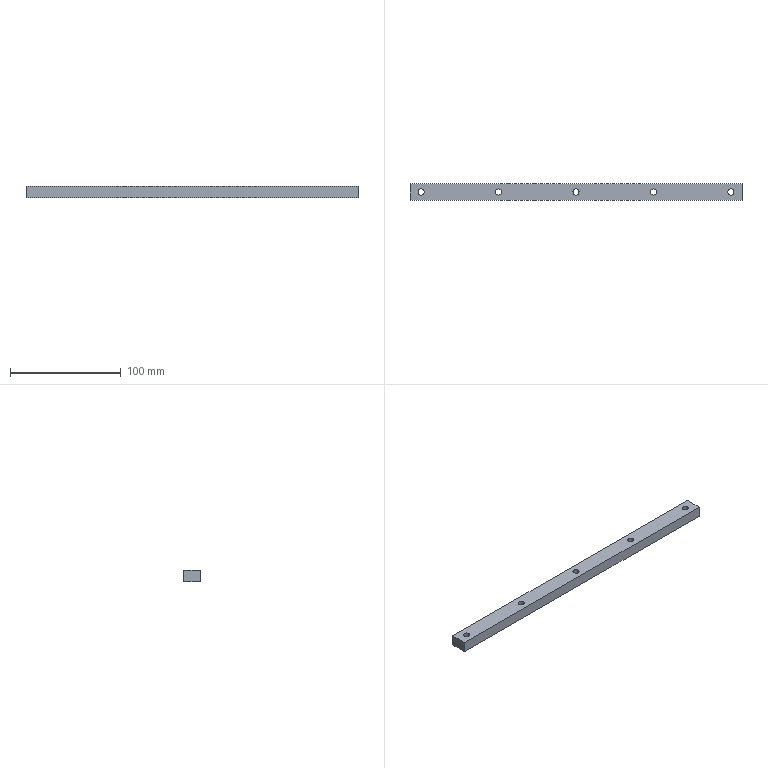Part | STEP file | Glass fixing plate | 1 solid | 31 faces | box 300 x 15 x 10 mm | volume 42251 mm3 | cylinder 20 | plane 11 | commonest cylinder face diameters 5.5 x10 10 x10